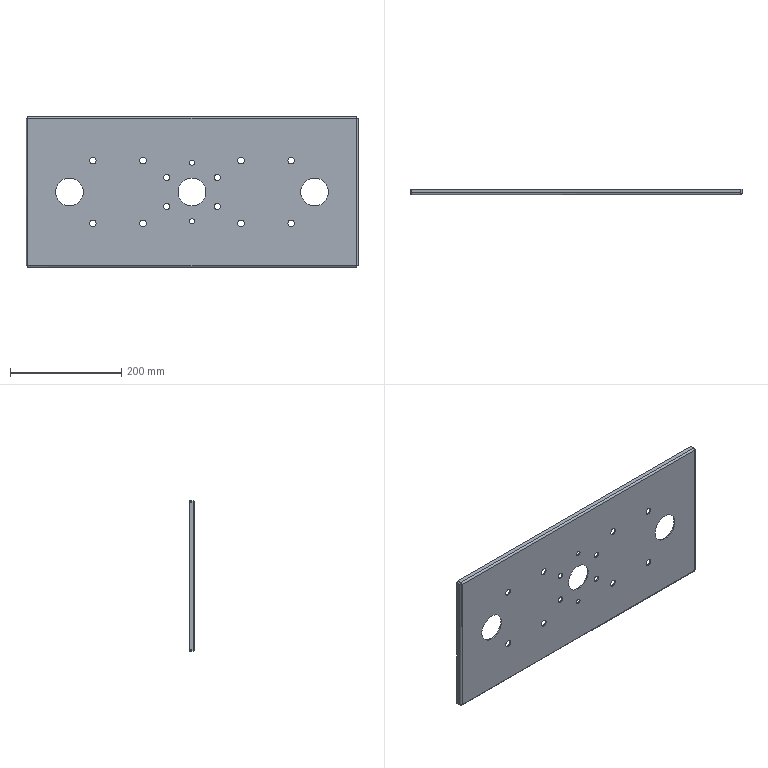Part | SolidWorks | features EdgeFlange 1, FlatPattern 1, ICE 1, SMBaseFlange 1, SheetMetal 1 | 1 solid | 72 faces | box 596 x 10 x 270 mm | volume 331666 mm3 | cylinder 42 | plane 22 | spline 8 | commonest cylinder face diameters 12 x16 11 x8 50 x6 2 x4 6 x4 9 x4